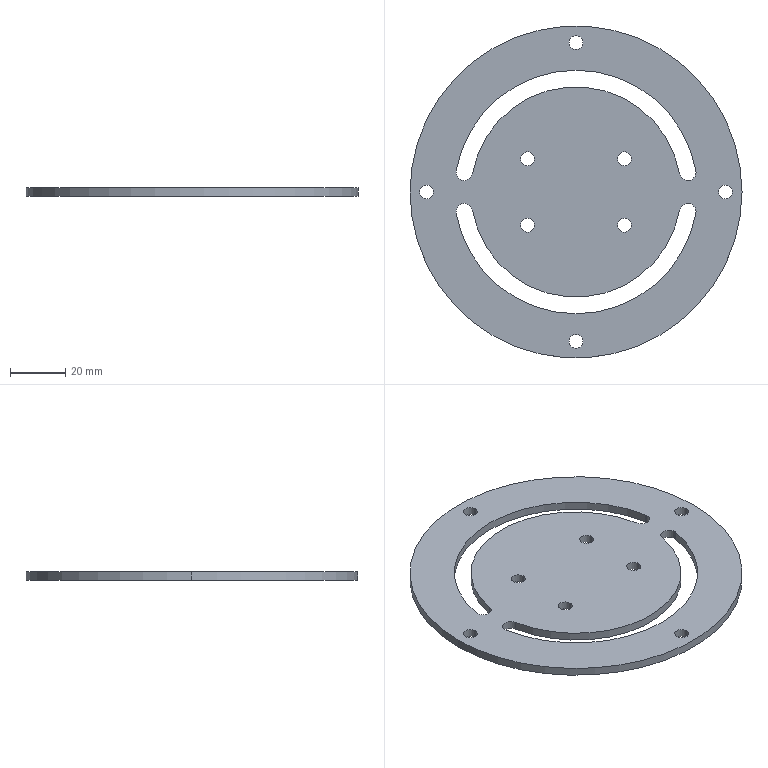Part | SolidWorks | features BaseBody 1 | 1 solid | 30 faces | box 120 x 120 x 3 mm | volume 29167 mm3 | cylinder 28 | plane 2 | commonest cylinder face diameters 5 x16 6 x6 76 x2 88 x2 120 x2
STEP:
#1=CARTESIAN_POINT('',(-60.,0.,3.));
#2=VERTEX_POINT('',#1);
#3=CARTESIAN_POINT('',(60.,0.,3.));
#4=VERTEX_POINT('',#3);
#5=CARTESIAN_POINT('',(0.,0.,3.));
#6=DIRECTION('',(0.,0.,-1.));
#7=DIRECTION('',(-1.,0.,0.));
#8=AXIS2_PLACEMENT_3D('',#5,#6,#7);
#9=CIRCLE('',#8,60.);
#10=EDGE_CURVE('',#2,#4,#9,.T.);
#11=ORIENTED_EDGE('',*,*,#10,.T.);
#12=CARTESIAN_POINT('',(60.,0.,0.));
#13=VERTEX_POINT('',#12);
#14=CARTESIAN_POINT('',(60.,0.,10.));
#15=DIRECTION('',(0.,0.,-1.));
#16=VECTOR('',#15,1000.);
#17=LINE('',#14,#16);
#18=EDGE_CURVE('',#4,#13,#17,.T.);
#19=ORIENTED_EDGE('',*,*,#18,.T.);
#20=CARTESIAN_POINT('',(-60.,0.,0.));
#21=VERTEX_POINT('',#20);
#22=CARTESIAN_POINT('',(0.,0.,0.));
#23=DIRECTION('',(0.,0.,-1.));
#24=DIRECTION('',(-1.,0.,0.));
#25=AXIS2_PLACEMENT_3D('',#22,#23,#24);
#26=CIRCLE('',#25,60.);
#27=EDGE_CURVE('',#21,#13,#26,.T.);
#28=ORIENTED_EDGE('',*,*,#27,.F.);
#29=CARTESIAN_POINT('',(-60.,0.,10.));
#30=DIRECTION('',(0.,0.,-1.));
#31=VECTOR('',#30,1000.);
#32=LINE('',#29,#31);
#33=EDGE_CURVE('',#2,#21,#32,.T.);
#34=ORIENTED_EDGE('',*,*,#33,.F.);
#35=EDGE_LOOP('',(#11,#19,#28,#34));
#36=FACE_OUTER_BOUND('',#35,.T.);
#37=CARTESIAN_POINT('',(0.,0.,10.));
#38=DIRECTION('',(0.,0.,-1.));
#39=DIRECTION('',(-1.,0.,0.));
#40=AXIS2_PLACEMENT_3D('',#37,#38,#39);
#41=CYLINDRICAL_SURFACE('',#40,60.);
#42=ADVANCED_FACE('',(#36),#41,.T.);
#43=CARTESIAN_POINT('',(43.377,7.12,0.));
#44=VERTEX_POINT('',#43);
#45=CARTESIAN_POINT('',(43.332,7.641,0.));
#46=VERTEX_POINT('',#45);
#47=CARTESIAN_POINT('',(40.377,7.12,0.));
#48=DIRECTION('',(0.,0.,1.));
#49=DIRECTION('',(1.,0.,0.));
#50=AXIS2_PLACEMENT_3D('',#47,#48,#49);
#51=CIRCLE('',#50,3.);
#52=EDGE_CURVE('',#44,#46,#51,.T.);
#53=ORIENTED_EDGE('',*,*,#52,.F.);
#54=CARTESIAN_POINT('',(43.377,7.12,3.));
#55=VERTEX_POINT('',#54);
#56=CARTESIAN_POINT('',(43.377,7.12,-7.));
#57=DIRECTION('',(0.,0.,1.));
#58=VECTOR('',#57,1000.);
#59=LINE('',#56,#58);
#60=EDGE_CURVE('',#44,#55,#59,.T.);
#61=ORIENTED_EDGE('',*,*,#60,.T.);
#62=CARTESIAN_POINT('',(43.332,7.641,3.));
#63=VERTEX_POINT('',#62);
#64=CARTESIAN_POINT('',(40.377,7.12,3.));
#65=DIRECTION('',(0.,0.,-1.));
#66=DIRECTION('',(1.,0.,0.));
#67=AXIS2_PLACEMENT_3D('',#64,#65,#66);
#68=CIRCLE('',#67,3.);
#69=EDGE_CURVE('',#63,#55,#68,.T.);
#70=ORIENTED_EDGE('',*,*,#69,.F.);
#71=CARTESIAN_POINT('',(43.332,7.641,-7.));
#72=DIRECTION('',(0.,0.,-1.));
#73=VECTOR('',#72,1000.);
#74=LINE('',#71,#73);
#75=EDGE_CURVE('',#63,#46,#74,.T.);
#76=ORIENTED_EDGE('',*,*,#75,.T.);
#77=EDGE_LOOP('',(#53,#61,#70,#76));
#78=FACE_OUTER_BOUND('',#77,.T.);
#79=CARTESIAN_POINT('',(40.377,7.12,-7.));
#80=DIRECTION('',(0.,0.,1.));
#81=DIRECTION('',(1.,0.,0.));
#82=AXIS2_PLACEMENT_3D('',#79,#80,#81);
#83=CYLINDRICAL_SURFACE('',#82,3.);
#84=ADVANCED_FACE('',(#78),#83,.F.);
#85=CARTESIAN_POINT('',(-15.,12.,3.));
#86=VERTEX_POINT('',#85);
#87=CARTESIAN_POINT('',(-20.,12.,3.));
#88=VERTEX_POINT('',#87);
#89=CARTESIAN_POINT('',(-17.5,12.,3.));
#90=DIRECTION('',(0.,0.,-1.));
#91=DIRECTION('',(-1.,0.,0.));
#92=AXIS2_PLACEMENT_3D('',#89,#90,#91);
#93=CIRCLE('',#92,2.5);
#94=EDGE_CURVE('',#86,#88,#93,.T.);
#95=ORIENTED_EDGE('',*,*,#94,.F.);
#96=CARTESIAN_POINT('',(-15.,12.,0.));
#97=VERTEX_POINT('',#96);
#98=CARTESIAN_POINT('',(-15.,12.,3.));
#99=DIRECTION('',(0.,0.,-1.));
#100=VECTOR('',#99,1000.);
#101=LINE('',#98,#100);
#102=EDGE_CURVE('',#86,#97,#101,.T.);
#103=ORIENTED_EDGE('',*,*,#102,.T.);
#104=CARTESIAN_POINT('',(-20.,12.,0.));
#105=VERTEX_POINT('',#104);
#106=CARTESIAN_POINT('',(-17.5,12.,0.));
#107=DIRECTION('',(0.,0.,1.));
#108=DIRECTION('',(-1.,0.,0.));
#109=AXIS2_PLACEMENT_3D('',#106,#107,#108);
#110=CIRCLE('',#109,2.5);
#111=EDGE_CURVE('',#105,#97,#110,.T.);
#112=ORIENTED_EDGE('',*,*,#111,.F.);
#113=CARTESIAN_POINT('',(-20.,12.,3.));
#114=DIRECTION('',(0.,0.,-1.));
#115=VECTOR('',#114,1000.);
#116=LINE('',#113,#115);
#117=EDGE_CURVE('',#88,#105,#116,.T.);
#118=ORIENTED_EDGE('',*,*,#117,.F.);
#119=EDGE_LOOP('',(#95,#103,#112,#118));
#120=FACE_OUTER_BOUND('',#119,.T.);
#121=CARTESIAN_POINT('',(-17.5,12.,3.));
#122=DIRECTION('',(0.,0.,-1.));
#123=DIRECTION('',(-1.,0.,0.));
#124=AXIS2_PLACEMENT_3D('',#121,#122,#123);
#125=CYLINDRICAL_SURFACE('',#124,2.5);
#126=ADVANCED_FACE('',(#120),#125,.F.);
#127=CARTESIAN_POINT('',(20.,-12.,3.));
#128=VERTEX_POINT('',#127);
#129=CARTESIAN_POINT('',(15.,-12.,3.));
#130=VERTEX_POINT('',#129);
#131=CARTESIAN_POINT('',(17.5,-12.,3.));
#132=DIRECTION('',(0.,0.,-1.));
#133=DIRECTION('',(-1.,0.,0.));
#134=AXIS2_PLACEMENT_3D('',#131,#132,#133);
#135=CIRCLE('',#134,2.5);
#136=EDGE_CURVE('',#128,#130,#135,.T.);
#137=ORIENTED_EDGE('',*,*,#136,.F.);
#138=CARTESIAN_POINT('',(20.,-12.,0.));
#139=VERTEX_POINT('',#138);
#140=CARTESIAN_POINT('',(20.,-12.,3.));
#141=DIRECTION('',(0.,0.,-1.));
#142=VECTOR('',#141,1000.);
#143=LINE('',#140,#142);
#144=EDGE_CURVE('',#128,#139,#143,.T.);
#145=ORIENTED_EDGE('',*,*,#144,.T.);
#146=CARTESIAN_POINT('',(15.,-12.,0.));
#147=VERTEX_POINT('',#146);
#148=CARTESIAN_POINT('',(17.5,-12.,0.));
#149=DIRECTION('',(0.,0.,1.));
#150=DIRECTION('',(-1.,0.,0.));
#151=AXIS2_PLACEMENT_3D('',#148,#149,#150);
#152=CIRCLE('',#151,2.5);
#153=EDGE_CURVE('',#147,#139,#152,.T.);
#154=ORIENTED_EDGE('',*,*,#153,.F.);
#155=CARTESIAN_POINT('',(15.,-12.,3.));
#156=DIRECTION('',(0.,0.,-1.));
#157=VECTOR('',#156,1000.);
#158=LINE('',#155,#157);
#159=EDGE_CURVE('',#130,#147,#158,.T.);
#160=ORIENTED_EDGE('',*,*,#159,.F.);
#161=EDGE_LOOP('',(#137,#145,#154,#160));
#162=FACE_OUTER_BOUND('',#161,.T.);
#163=CARTESIAN_POINT('',(17.5,-12.,3.));
#164=DIRECTION('',(0.,0.,-1.));
#165=DIRECTION('',(-1.,0.,0.));
#166=AXIS2_PLACEMENT_3D('',#163,#164,#165);
#167=CYLINDRICAL_SURFACE('',#166,2.5);
#168=ADVANCED_FACE('',(#162),#167,.F.);
#169=CARTESIAN_POINT('',(-51.5,0.,3.));
#170=VERTEX_POINT('',#169);
#171=CARTESIAN_POINT('',(-56.5,0.,3.));
#172=VERTEX_POINT('',#171);
#173=CARTESIAN_POINT('',(-54.,0.,3.));
#174=DIRECTION('',(0.,0.,-1.));
#175=DIRECTION('',(-1.,0.,0.));
#176=AXIS2_PLACEMENT_3D('',#173,#174,#175);
#177=CIRCLE('',#176,2.5);
#178=EDGE_CURVE('',#170,#172,#177,.T.);
#179=ORIENTED_EDGE('',*,*,#178,.F.);
#180=CARTESIAN_POINT('',(-51.5,0.,0.));
#181=VERTEX_POINT('',#180);
#182=CARTESIAN_POINT('',(-51.5,0.,3.));
#183=DIRECTION('',(0.,0.,-1.));
#184=VECTOR('',#183,1000.);
#185=LINE('',#182,#184);
#186=EDGE_CURVE('',#170,#181,#185,.T.);
#187=ORIENTED_EDGE('',*,*,#186,.T.);
#188=CARTESIAN_POINT('',(-56.5,0.,0.));
#189=VERTEX_POINT('',#188);
#190=CARTESIAN_POINT('',(-54.,0.,0.));
#191=DIRECTION('',(0.,0.,1.));
#192=DIRECTION('',(-1.,0.,0.));
#193=AXIS2_PLACEMENT_3D('',#190,#191,#192);
#194=CIRCLE('',#193,2.5);
#195=EDGE_CURVE('',#189,#181,#194,.T.);
#196=ORIENTED_EDGE('',*,*,#195,.F.);
#197=CARTESIAN_POINT('',(-56.5,0.,3.));
#198=DIRECTION('',(0.,0.,-1.));
#199=VECTOR('',#198,1000.);
#200=LINE('',#197,#199);
#201=EDGE_CURVE('',#172,#189,#200,.T.);
#202=ORIENTED_EDGE('',*,*,#201,.F.);
#203=EDGE_LOOP('',(#179,#187,#196,#202));
#204=FACE_OUTER_BOUND('',#203,.T.);
#205=CARTESIAN_POINT('',(-54.,0.,3.));
#206=DIRECTION('',(0.,0.,-1.));
#207=DIRECTION('',(-1.,0.,0.));
#208=AXIS2_PLACEMENT_3D('',#205,#206,#207);
#209=CYLINDRICAL_SURFACE('',#208,2.5);
#210=ADVANCED_FACE('',(#204),#209,.F.);
#211=CARTESIAN_POINT('',(56.5,0.,3.));
#212=VERTEX_POINT('',#211);
#213=CARTESIAN_POINT('',(51.5,0.,3.));
#214=VERTEX_POINT('',#213);
#215=CARTESIAN_POINT('',(54.,0.,3.));
#216=DIRECTION('',(0.,0.,-1.));
#217=DIRECTION('',(-1.,0.,0.));
#218=AXIS2_PLACEMENT_3D('',#215,#216,#217);
#219=CIRCLE('',#218,2.5);
#220=EDGE_CURVE('',#212,#214,#219,.T.);
#221=ORIENTED_EDGE('',*,*,#220,.F.);
#222=CARTESIAN_POINT('',(56.5,0.,0.));
#223=VERTEX_POINT('',#222);
#224=CARTESIAN_POINT('',(56.5,0.,3.));
#225=DIRECTION('',(0.,0.,-1.));
#226=VECTOR('',#225,1000.);
#227=LINE('',#224,#226);
#228=EDGE_CURVE('',#212,#223,#227,.T.);
#229=ORIENTED_EDGE('',*,*,#228,.T.);
#230=CARTESIAN_POINT('',(51.5,0.,0.));
#231=VERTEX_POINT('',#230);
#232=CARTESIAN_POINT('',(54.,0.,0.));
#233=DIRECTION('',(0.,0.,1.));
#234=DIRECTION('',(-1.,0.,0.));
#235=AXIS2_PLACEMENT_3D('',#232,#233,#234);
#236=CIRCLE('',#235,2.5);
#237=EDGE_CURVE('',#231,#223,#236,.T.);
#238=ORIENTED_EDGE('',*,*,#237,.F.);
#239=CARTESIAN_POINT('',(51.5,0.,3.));
#240=DIRECTION('',(0.,0.,-1.));
#241=VECTOR('',#240,1000.);
#242=LINE('',#239,#241);
#243=EDGE_CURVE('',#214,#231,#242,.T.);
#244=ORIENTED_EDGE('',*,*,#243,.F.);
#245=EDGE_LOOP('',(#221,#229,#238,#244));
#246=FACE_OUTER_BOUND('',#245,.T.);
#247=CARTESIAN_POINT('',(54.,0.,3.));
#248=DIRECTION('',(0.,0.,-1.));
#249=DIRECTION('',(-1.,0.,0.));
#250=AXIS2_PLACEMENT_3D('',#247,#248,#249);
#251=CYLINDRICAL_SURFACE('',#250,2.5);
#252=ADVANCED_FACE('',(#246),#251,.F.);
#253=CARTESIAN_POINT('',(2.5,54.,3.));
#254=VERTEX_POINT('',#253);
#255=CARTESIAN_POINT('',(-2.5,54.,3.));
#256=VERTEX_POINT('',#255);
#257=CARTESIAN_POINT('',(0.,54.,3.));
#258=DIRECTION('',(0.,0.,-1.));
#259=DIRECTION('',(-1.,0.,0.));
#260=AXIS2_PLACEMENT_3D('',#257,#258,#259);
#261=CIRCLE('',#260,2.5);
#262=EDGE_CURVE('',#254,#256,#261,.T.);
#263=ORIENTED_EDGE('',*,*,#262,.F.);
#264=CARTESIAN_POINT('',(2.5,54.,0.));
#265=VERTEX_POINT('',#264);
#266=CARTESIAN_POINT('',(2.5,54.,3.));
#267=DIRECTION('',(0.,0.,-1.));
#268=VECTOR('',#267,1000.);
#269=LINE('',#266,#268);
#270=EDGE_CURVE('',#254,#265,#269,.T.);
#271=ORIENTED_EDGE('',*,*,#270,.T.);
#272=CARTESIAN_POINT('',(-2.5,54.,0.));
#273=VERTEX_POINT('',#272);
#274=CARTESIAN_POINT('',(0.,54.,0.));
#275=DIRECTION('',(0.,0.,1.));
#276=DIRECTION('',(-1.,0.,0.));
#277=AXIS2_PLACEMENT_3D('',#274,#275,#276);
#278=CIRCLE('',#277,2.5);
#279=EDGE_CURVE('',#273,#265,#278,.T.);
#280=ORIENTED_EDGE('',*,*,#279,.F.);
#281=CARTESIAN_POINT('',(-2.5,54.,3.));
#282=DIRECTION('',(0.,0.,-1.));
#283=VECTOR('',#282,1000.);
#284=LINE('',#281,#283);
#285=EDGE_CURVE('',#256,#273,#284,.T.);
#286=ORIENTED_EDGE('',*,*,#285,.F.);
#287=EDGE_LOOP('',(#263,#271,#280,#286));
#288=FACE_OUTER_BOUND('',#287,.T.);
#289=CARTESIAN_POINT('',(0.,54.,3.));
#290=DIRECTION('',(0.,0.,-1.));
#291=DIRECTION('',(-1.,0.,0.));
#292=AXIS2_PLACEMENT_3D('',#289,#290,#291);
#293=CYLINDRICAL_SURFACE('',#292,2.5);
#294=ADVANCED_FACE('',(#288),#293,.F.);
#295=CARTESIAN_POINT('',(2.5,-54.,3.));
#296=VERTEX_POINT('',#295);
#297=CARTESIAN_POINT('',(-2.5,-54.,3.));
#298=VERTEX_POINT('',#297);
#299=CARTESIAN_POINT('',(0.,-54.,3.));
#300=DIRECTION('',(0.,0.,-1.));
#301=DIRECTION('',(-1.,0.,0.));
#302=AXIS2_PLACEMENT_3D('',#299,#300,#301);
#303=CIRCLE('',#302,2.5);
#304=EDGE_CURVE('',#296,#298,#303,.T.);
#305=ORIENTED_EDGE('',*,*,#304,.F.);
#306=CARTESIAN_POINT('',(2.5,-54.,0.));
#307=VERTEX_POINT('',#306);
#308=CARTESIAN_POINT('',(2.5,-54.,3.));
#309=DIRECTION('',(0.,0.,-1.));
#310=VECTOR('',#309,1000.);
#311=LINE('',#308,#310);
#312=EDGE_CURVE('',#296,#307,#311,.T.);
#313=ORIENTED_EDGE('',*,*,#312,.T.);
#314=CARTESIAN_POINT('',(-2.5,-54.,0.));
#315=VERTEX_POINT('',#314);
#316=CARTESIAN_POINT('',(0.,-54.,0.));
#317=DIRECTION('',(0.,0.,1.));
#318=DIRECTION('',(-1.,0.,0.));
#319=AXIS2_PLACEMENT_3D('',#316,#317,#318);
#320=CIRCLE('',#319,2.5);
#321=EDGE_CURVE('',#315,#307,#320,.T.);
#322=ORIENTED_EDGE('',*,*,#321,.F.);
#323=CARTESIAN_POINT('',(-2.5,-54.,3.));
#324=DIRECTION('',(0.,0.,-1.));
#325=VECTOR('',#324,1000.);
#326=LINE('',#323,#325);
#327=EDGE_CURVE('',#298,#315,#326,.T.);
#328=ORIENTED_EDGE('',*,*,#327,.F.);
#329=EDGE_LOOP('',(#305,#313,#322,#328));
#330=FACE_OUTER_BOUND('',#329,.T.);
#331=CARTESIAN_POINT('',(0.,-54.,3.));
#332=DIRECTION('',(0.,0.,-1.));
#333=DIRECTION('',(-1.,0.,0.));
#334=AXIS2_PLACEMENT_3D('',#331,#332,#333);
#335=CYLINDRICAL_SURFACE('',#334,2.5);
#336=ADVANCED_FACE('',(#330),#335,.F.);
#337=CARTESIAN_POINT('',(20.,12.,3.));
#338=VERTEX_POINT('',#337);
#339=CARTESIAN_POINT('',(15.,12.,3.));
#340=VERTEX_POINT('',#339);
#341=CARTESIAN_POINT('',(17.5,12.,3.));
#342=DIRECTION('',(0.,0.,-1.));
#343=DIRECTION('',(-1.,0.,0.));
#344=AXIS2_PLACEMENT_3D('',#341,#342,#343);
#345=CIRCLE('',#344,2.5);
#346=EDGE_CURVE('',#338,#340,#345,.T.);
#347=ORIENTED_EDGE('',*,*,#346,.F.);
#348=CARTESIAN_POINT('',(20.,12.,0.));
#349=VERTEX_POINT('',#348);
#350=CARTESIAN_POINT('',(20.,12.,3.));
#351=DIRECTION('',(0.,0.,-1.));
#352=VECTOR('',#351,1000.);
#353=LINE('',#350,#352);
#354=EDGE_CURVE('',#338,#349,#353,.T.);
#355=ORIENTED_EDGE('',*,*,#354,.T.);
#356=CARTESIAN_POINT('',(15.,12.,0.));
#357=VERTEX_POINT('',#356);
#358=CARTESIAN_POINT('',(17.5,12.,0.));
#359=DIRECTION('',(0.,0.,1.));
#360=DIRECTION('',(-1.,0.,0.));
#361=AXIS2_PLACEMENT_3D('',#358,#359,#360);
#362=CIRCLE('',#361,2.5);
#363=EDGE_CURVE('',#357,#349,#362,.T.);
#364=ORIENTED_EDGE('',*,*,#363,.F.);
#365=CARTESIAN_POINT('',(15.,12.,3.));
#366=DIRECTION('',(0.,0.,-1.));
#367=VECTOR('',#366,1000.);
#368=LINE('',#365,#367);
#369=EDGE_CURVE('',#340,#357,#368,.T.);
#370=ORIENTED_EDGE('',*,*,#369,.F.);
#371=EDGE_LOOP('',(#347,#355,#364,#370));
#372=FACE_OUTER_BOUND('',#371,.T.);
#373=CARTESIAN_POINT('',(17.5,12.,3.));
#374=DIRECTION('',(0.,0.,-1.));
#375=DIRECTION('',(-1.,0.,0.));
#376=AXIS2_PLACEMENT_3D('',#373,#374,#375);
#377=CYLINDRICAL_SURFACE('',#376,2.5);
#378=ADVANCED_FACE('',(#372),#377,.F.);
#379=CARTESIAN_POINT('',(-15.,-12.,3.));
#380=VERTEX_POINT('',#379);
#381=CARTESIAN_POINT('',(-20.,-12.,3.));
#382=VERTEX_POINT('',#381);
#383=CARTESIAN_POINT('',(-17.5,-12.,3.));
#384=DIRECTION('',(0.,0.,-1.));
#385=DIRECTION('',(-1.,0.,0.));
#386=AXIS2_PLACEMENT_3D('',#383,#384,#385);
#387=CIRCLE('',#386,2.5);
#388=EDGE_CURVE('',#380,#382,#387,.T.);
#389=ORIENTED_EDGE('',*,*,#388,.F.);
#390=CARTESIAN_POINT('',(-15.,-12.,0.));
#391=VERTEX_POINT('',#390);
#392=CARTESIAN_POINT('',(-15.,-12.,3.));
#393=DIRECTION('',(0.,0.,-1.));
#394=VECTOR('',#393,1000.);
#395=LINE('',#392,#394);
#396=EDGE_CURVE('',#380,#391,#395,.T.);
#397=ORIENTED_EDGE('',*,*,#396,.T.);
#398=CARTESIAN_POINT('',(-20.,-12.,0.));
#399=VERTEX_POINT('',#398);
#400=CARTESIAN_POINT('',(-17.5,-12.,0.));
#401=DIRECTION('',(0.,0.,1.));
#402=DIRECTION('',(-1.,0.,0.));
#403=AXIS2_PLACEMENT_3D('',#400,#401,#402);
#404=CIRCLE('',#403,2.5);
#405=EDGE_CURVE('',#399,#391,#404,.T.);
#406=ORIENTED_EDGE('',*,*,#405,.F.);
#407=CARTESIAN_POINT('',(-20.,-12.,3.));
#408=DIRECTION('',(0.,0.,-1.));
#409=VECTOR('',#408,1000.);
#410=LINE('',#407,#409);
#411=EDGE_CURVE('',#382,#399,#410,.T.);
#412=ORIENTED_EDGE('',*,*,#411,.F.);
#413=EDGE_LOOP('',(#389,#397,#406,#412));
#414=FACE_OUTER_BOUND('',#413,.T.);
#415=CARTESIAN_POINT('',(-17.5,-12.,3.));
#416=DIRECTION('',(0.,0.,-1.));
#417=DIRECTION('',(-1.,0.,0.));
#418=AXIS2_PLACEMENT_3D('',#415,#416,#417);
#419=CYLINDRICAL_SURFACE('',#418,2.5);
#420=ADVANCED_FACE('',(#414),#419,.F.);
#421=CARTESIAN_POINT('',(43.377,-7.12,0.));
#422=VERTEX_POINT('',#421);
#423=CARTESIAN_POINT('',(37.423,-6.599,0.));
#424=VERTEX_POINT('',#423);
#425=CARTESIAN_POINT('',(40.377,-7.12,0.));
#426=DIRECTION('',(0.,0.,1.));
#427=DIRECTION('',(1.,0.,0.));
#428=AXIS2_PLACEMENT_3D('',#425,#426,#427);
#429=CIRCLE('',#428,3.);
#430=EDGE_CURVE('',#422,#424,#429,.T.);
#431=ORIENTED_EDGE('',*,*,#430,.F.);
#432=CARTESIAN_POINT('',(43.377,-7.12,3.));
#433=VERTEX_POINT('',#432);
#434=CARTESIAN_POINT('',(43.377,-7.12,-7.));
#435=DIRECTION('',(0.,0.,1.));
#436=VECTOR('',#435,1000.);
#437=LINE('',#434,#436);
#438=EDGE_CURVE('',#422,#433,#437,.T.);
#439=ORIENTED_EDGE('',*,*,#438,.T.);
#440=CARTESIAN_POINT('',(37.423,-6.599,3.));
#441=VERTEX_POINT('',#440);
#442=CARTESIAN_POINT('',(40.377,-7.12,3.));
#443=DIRECTION('',(0.,0.,-1.));
#444=DIRECTION('',(1.,0.,0.));
#445=AXIS2_PLACEMENT_3D('',#442,#443,#444);
#446=CIRCLE('',#445,3.);
#447=EDGE_CURVE('',#441,#433,#446,.T.);
#448=ORIENTED_EDGE('',*,*,#447,.F.);
#449=CARTESIAN_POINT('',(37.423,-6.599,-7.));
#450=DIRECTION('',(0.,0.,1.));
#451=VECTOR('',#450,1000.);
#452=LINE('',#449,#451);
#453=EDGE_CURVE('',#424,#441,#452,.T.);
#454=ORIENTED_EDGE('',*,*,#453,.F.);
#455=EDGE_LOOP('',(#431,#439,#448,#454));
#456=FACE_OUTER_BOUND('',#455,.T.);
#457=CARTESIAN_POINT('',(40.377,-7.12,-7.));
#458=DIRECTION('',(0.,0.,1.));
#459=DIRECTION('',(1.,0.,0.));
#460=AXIS2_PLACEMENT_3D('',#457,#458,#459);
#461=CYLINDRICAL_SURFACE('',#460,3.);
#462=ADVANCED_FACE('',(#456),#461,.F.);
#463=ORIENTED_EDGE('',*,*,#27,.T.);
#464=CARTESIAN_POINT('',(0.,0.,0.));
#465=DIRECTION('',(0.,0.,-1.));
#466=DIRECTION('',(-1.,0.,0.));
#467=AXIS2_PLACEMENT_3D('',#464,#465,#466);
#468=CIRCLE('',#467,60.);
#469=EDGE_CURVE('',#13,#21,#468,.T.);
#470=ORIENTED_EDGE('',*,*,#469,.T.);
#471=EDGE_LOOP('',(#463,#470));
#472=FACE_OUTER_BOUND('',#471,.T.);
#473=CARTESIAN_POINT('',(-37.423,6.599,0.));
#474=VERTEX_POINT('',#473);
#475=CARTESIAN_POINT('',(37.423,6.599,0.));
#476=VERTEX_POINT('',#475);
#477=CARTESIAN_POINT('',(0.,0.,0.));
#478=DIRECTION('',(0.,0.,-1.));
#479=DIRECTION('',(1.,0.,0.));
#480=AXIS2_PLACEMENT_3D('',#477,#478,#479);
#481=CIRCLE('',#480,38.);
#482=EDGE_CURVE('',#474,#476,#481,.T.);
#483=ORIENTED_EDGE('',*,*,#482,.T.);
#484=CARTESIAN_POINT('',(40.377,7.12,0.));
#485=DIRECTION('',(0.,0.,1.));
#486=DIRECTION('',(1.,0.,0.));
#487=AXIS2_PLACEMENT_3D('',#484,#485,#486);
#488=CIRCLE('',#487,3.);
#489=EDGE_CURVE('',#476,#44,#488,.T.);
#490=ORIENTED_EDGE('',*,*,#489,.T.);
#491=ORIENTED_EDGE('',*,*,#52,.T.);
#492=CARTESIAN_POINT('',(-43.332,7.641,0.));
#493=VERTEX_POINT('',#492);
#494=CARTESIAN_POINT('',(0.,0.,0.));
#495=DIRECTION('',(0.,0.,1.));
#496=DIRECTION('',(1.,0.,0.));
#497=AXIS2_PLACEMENT_3D('',#494,#495,#496);
#498=CIRCLE('',#497,44.);
#499=EDGE_CURVE('',#46,#493,#498,.T.);
#500=ORIENTED_EDGE('',*,*,#499,.T.);
#501=CARTESIAN_POINT('',(-40.377,7.12,0.));
#502=DIRECTION('',(0.,0.,1.));
#503=DIRECTION('',(1.,0.,0.));
#504=AXIS2_PLACEMENT_3D('',#501,#502,#503);
#505=CIRCLE('',#504,3.);
#506=EDGE_CURVE('',#493,#474,#505,.T.);
#507=ORIENTED_EDGE('',*,*,#506,.T.);
#508=EDGE_LOOP('',(#483,#490,#491,#500,#507));
#509=FACE_BOUND('',#508,.T.);
#510=ORIENTED_EDGE('',*,*,#111,.T.);
#511=CARTESIAN_POINT('',(-17.5,12.,0.));
#512=DIRECTION('',(0.,0.,1.));
#513=DIRECTION('',(-1.,0.,0.));
#514=AXIS2_PLACEMENT_3D('',#511,#512,#513);
#515=CIRCLE('',#514,2.5);
#516=EDGE_CURVE('',#97,#105,#515,.T.);
#517=ORIENTED_EDGE('',*,*,#516,.T.);
#518=EDGE_LOOP('',(#510,#517));
#519=FACE_BOUND('',#518,.T.);
#520=ORIENTED_EDGE('',*,*,#153,.T.);
#521=CARTESIAN_POINT('',(17.5,-12.,0.));
#522=DIRECTION('',(0.,0.,1.));
#523=DIRECTION('',(-1.,0.,0.));
#524=AXIS2_PLACEMENT_3D('',#521,#522,#523);
#525=CIRCLE('',#524,2.5);
#526=EDGE_CURVE('',#139,#147,#525,.T.);
#527=ORIENTED_EDGE('',*,*,#526,.T.);
#528=EDGE_LOOP('',(#520,#527));
#529=FACE_BOUND('',#528,.T.);
#530=ORIENTED_EDGE('',*,*,#195,.T.);
#531=CARTESIAN_POINT('',(-54.,0.,0.));
#532=DIRECTION('',(0.,0.,1.));
#533=DIRECTION('',(-1.,0.,0.));
#534=AXIS2_PLACEMENT_3D('',#531,#532,#533);
#535=CIRCLE('',#534,2.5);
#536=EDGE_CURVE('',#181,#189,#535,.T.);
#537=ORIENTED_EDGE('',*,*,#536,.T.);
#538=EDGE_LOOP('',(#530,#537));
#539=FACE_BOUND('',#538,.T.);
#540=ORIENTED_EDGE('',*,*,#237,.T.);
#541=CARTESIAN_POINT('',(54.,0.,0.));
#542=DIRECTION('',(0.,0.,1.));
#543=DIRECTION('',(-1.,0.,0.));
#544=AXIS2_PLACEMENT_3D('',#541,#542,#543);
#545=CIRCLE('',#544,2.5);
#546=EDGE_CURVE('',#223,#231,#545,.T.);
#547=ORIENTED_EDGE('',*,*,#546,.T.);
#548=EDGE_LOOP('',(#540,#547));
#549=FACE_BOUND('',#548,.T.);
#550=ORIENTED_EDGE('',*,*,#279,.T.);
#551=CARTESIAN_POINT('',(0.,54.,0.));
#552=DIRECTION('',(0.,0.,1.));
#553=DIRECTION('',(-1.,0.,0.));
#554=AXIS2_PLACEMENT_3D('',#551,#552,#553);
#555=CIRCLE('',#554,2.5);
#556=EDGE_CURVE('',#265,#273,#555,.T.);
#557=ORIENTED_EDGE('',*,*,#556,.T.);
#558=EDGE_LOOP('',(#550,#557));
#559=FACE_BOUND('',#558,.T.);
#560=ORIENTED_EDGE('',*,*,#321,.T.);
#561=CARTESIAN_POINT('',(0.,-54.,0.));
#562=DIRECTION('',(0.,0.,1.));
#563=DIRECTION('',(-1.,0.,0.));
#564=AXIS2_PLACEMENT_3D('',#561,#562,#563);
#565=CIRCLE('',#564,2.5);
#566=EDGE_CURVE('',#307,#315,#565,.T.);
#567=ORIENTED_EDGE('',*,*,#566,.T.);
#568=EDGE_LOOP('',(#560,#567));
#569=FACE_BOUND('',#568,.T.);
#570=ORIENTED_EDGE('',*,*,#363,.T.);
#571=CARTESIAN_POINT('',(17.5,12.,0.));
#572=DIRECTION('',(0.,0.,1.));
#573=DIRECTION('',(-1.,0.,0.));
#574=AXIS2_PLACEMENT_3D('',#571,#572,#573);
#575=CIRCLE('',#574,2.5);
#576=EDGE_CURVE('',#349,#357,#575,.T.);
#577=ORIENTED_EDGE('',*,*,#576,.T.);
#578=EDGE_LOOP('',(#570,#577));
#579=FACE_BOUND('',#578,.T.);
#580=ORIENTED_EDGE('',*,*,#405,.T.);
#581=CARTESIAN_POINT('',(-17.5,-12.,0.));
#582=DIRECTION('',(0.,0.,1.));
#583=DIRECTION('',(-1.,0.,0.));
#584=AXIS2_PLACEMENT_3D('',#581,#582,#583);
#585=CIRCLE('',#584,2.5);
#586=EDGE_CURVE('',#391,#399,#585,.T.);
#587=ORIENTED_EDGE('',*,*,#586,.T.);
#588=EDGE_LOOP('',(#580,#587));
#589=FACE_BOUND('',#588,.T.);
#590=CARTESIAN_POINT('',(-43.332,-7.641,0.));
#591=VERTEX_POINT('',#590);
#592=CARTESIAN_POINT('',(43.332,-7.641,0.));
#593=VERTEX_POINT('',#592);
#594=CARTESIAN_POINT('',(0.,0.,0.));
#595=DIRECTION('',(0.,0.,1.));
#596=DIRECTION('',(1.,0.,0.));
#597=AXIS2_PLACEMENT_3D('',#594,#595,#596);
#598=CIRCLE('',#597,44.);
#599=EDGE_CURVE('',#591,#593,#598,.T.);
#600=ORIENTED_EDGE('',*,*,#599,.T.);
#601=CARTESIAN_POINT('',(40.377,-7.12,0.));
#602=DIRECTION('',(0.,0.,1.));
#603=DIRECTION('',(1.,0.,0.));
#604=AXIS2_PLACEMENT_3D('',#601,#602,#603);
#605=CIRCLE('',#604,3.);
#606=EDGE_CURVE('',#593,#422,#605,.T.);
#607=ORIENTED_EDGE('',*,*,#606,.T.);
#608=ORIENTED_EDGE('',*,*,#430,.T.);
#609=CARTESIAN_POINT('',(-37.423,-6.599,0.));
#610=VERTEX_POINT('',#609);
#611=CARTESIAN_POINT('',(0.,0.,0.));
#612=DIRECTION('',(0.,0.,-1.));
#613=DIRECTION('',(1.,0.,0.));
#614=AXIS2_PLACEMENT_3D('',#611,#612,#613);
#615=CIRCLE('',#614,38.);
#616=EDGE_CURVE('',#424,#610,#615,.T.);
#617=ORIENTED_EDGE('',*,*,#616,.T.);
#618=CARTESIAN_POINT('',(-40.377,-7.12,0.));
#619=DIRECTION('',(0.,0.,1.));
#620=DIRECTION('',(1.,0.,0.));
#621=AXIS2_PLACEMENT_3D('',#618,#619,#620);
#622=CIRCLE('',#621,3.);
#623=EDGE_CURVE('',#610,#591,#622,.T.);
#624=ORIENTED_EDGE('',*,*,#623,.T.);
#625=EDGE_LOOP('',(#600,#607,#608,#617,#624));
#626=FACE_BOUND('',#625,.T.);
#627=CARTESIAN_POINT('',(0.,0.,0.));
#628=DIRECTION('',(0.,0.,-1.));
#629=DIRECTION('',(-1.,0.,0.));
#630=AXIS2_PLACEMENT_3D('',#627,#628,#629);
#631=PLANE('',#630);
#632=ADVANCED_FACE('',(#472,#509,#519,#529,#539,#549,#559,#569,#579,#589,#626),#631,.T.);
#633=ORIENTED_EDGE('',*,*,#18,.F.);
#634=CARTESIAN_POINT('',(0.,0.,3.));
#635=DIRECTION('',(0.,0.,-1.));
#636=DIRECTION('',(-1.,0.,0.));
#637=AXIS2_PLACEMENT_3D('',#634,#635,#636);
#638=CIRCLE('',#637,60.);
#639=EDGE_CURVE('',#4,#2,#638,.T.);
#640=ORIENTED_EDGE('',*,*,#639,.T.);
#641=ORIENTED_EDGE('',*,*,#33,.T.);
#642=ORIENTED_EDGE('',*,*,#469,.F.);
#643=EDGE_LOOP('',(#633,#640,#641,#642));
#644=FACE_OUTER_BOUND('',#643,.T.);
#645=CARTESIAN_POINT('',(0.,0.,10.));
#646=DIRECTION('',(0.,0.,-1.));
#647=DIRECTION('',(-1.,0.,0.));
#648=AXIS2_PLACEMENT_3D('',#645,#646,#647);
#649=CYLINDRICAL_SURFACE('',#648,60.);
#650=ADVANCED_FACE('',(#644),#649,.T.);
#651=ORIENTED_EDGE('',*,*,#60,.F.);
#652=ORIENTED_EDGE('',*,*,#489,.F.);
#653=CARTESIAN_POINT('',(37.423,6.599,3.));
#654=VERTEX_POINT('',#653);
#655=CARTESIAN_POINT('',(37.423,6.599,-7.));
#656=DIRECTION('',(0.,0.,-1.));
#657=VECTOR('',#656,1000.);
#658=LINE('',#655,#657);
#659=EDGE_CURVE('',#654,#476,#658,.T.);
#660=ORIENTED_EDGE('',*,*,#659,.F.);
#661=CARTESIAN_POINT('',(40.377,7.12,3.));
#662=DIRECTION('',(0.,0.,-1.));
#663=DIRECTION('',(1.,0.,0.));
#664=AXIS2_PLACEMENT_3D('',#661,#662,#663);
#665=CIRCLE('',#664,3.);
#666=EDGE_CURVE('',#55,#654,#665,.T.);
#667=ORIENTED_EDGE('',*,*,#666,.F.);
#668=EDGE_LOOP('',(#651,#652,#660,#667));
#669=FACE_OUTER_BOUND('',#668,.T.);
#670=CARTESIAN_POINT('',(40.377,7.12,-7.));
#671=DIRECTION('',(0.,0.,1.));
#672=DIRECTION('',(1.,0.,0.));
#673=AXIS2_PLACEMENT_3D('',#670,#671,#672);
#674=CYLINDRICAL_SURFACE('',#673,3.);
#675=ADVANCED_FACE('',(#669),#674,.F.);
#676=CARTESIAN_POINT('',(-37.423,6.599,3.));
#677=VERTEX_POINT('',#676);
#678=CARTESIAN_POINT('',(0.,0.,3.));
#679=DIRECTION('',(0.,0.,-1.));
#680=DIRECTION('',(1.,0.,0.));
#681=AXIS2_PLACEMENT_3D('',#678,#679,#680);
#682=CIRCLE('',#681,38.);
#683=EDGE_CURVE('',#677,#654,#682,.T.);
#684=ORIENTED_EDGE('',*,*,#683,.T.);
#685=ORIENTED_EDGE('',*,*,#659,.T.);
#686=ORIENTED_EDGE('',*,*,#482,.F.);
#687=CARTESIAN_POINT('',(-37.423,6.599,-7.));
#688=DIRECTION('',(0.,0.,1.));
#689=VECTOR('',#688,1000.);
#690=LINE('',#687,#689);
#691=EDGE_CURVE('',#474,#677,#690,.T.);
#692=ORIENTED_EDGE('',*,*,#691,.T.);
#693=EDGE_LOOP('',(#684,#685,#686,#692));
#694=FACE_OUTER_BOUND('',#693,.T.);
#695=CARTESIAN_POINT('',(0.,0.,-7.));
#696=DIRECTION('',(0.,0.,1.));
#697=DIRECTION('',(1.,0.,0.));
#698=AXIS2_PLACEMENT_3D('',#695,#696,#697);
#699=CYLINDRICAL_SURFACE('',#698,38.);
#700=ADVANCED_FACE('',(#694),#699,.T.);
#701=CARTESIAN_POINT('',(-43.332,7.641,3.));
#702=VERTEX_POINT('',#701);
#703=CARTESIAN_POINT('',(-43.332,7.641,-7.));
#704=DIRECTION('',(0.,0.,-1.));
#705=VECTOR('',#704,1000.);
#706=LINE('',#703,#705);
#707=EDGE_CURVE('',#702,#493,#706,.T.);
#708=ORIENTED_EDGE('',*,*,#707,.F.);
#709=CARTESIAN_POINT('',(-40.377,7.12,3.));
#710=DIRECTION('',(0.,0.,-1.));
#711=DIRECTION('',(1.,0.,0.));
#712=AXIS2_PLACEMENT_3D('',#709,#710,#711);
#713=CIRCLE('',#712,3.);
#714=EDGE_CURVE('',#677,#702,#713,.T.);
#715=ORIENTED_EDGE('',*,*,#714,.F.);
#716=ORIENTED_EDGE('',*,*,#691,.F.);
#717=ORIENTED_EDGE('',*,*,#506,.F.);
#718=EDGE_LOOP('',(#708,#715,#716,#717));
#719=FACE_OUTER_BOUND('',#718,.T.);
#720=CARTESIAN_POINT('',(-40.377,7.12,-7.));
#721=DIRECTION('',(0.,0.,1.));
#722=DIRECTION('',(1.,0.,0.));
#723=AXIS2_PLACEMENT_3D('',#720,#721,#722);
#724=CYLINDRICAL_SURFACE('',#723,3.);
#725=ADVANCED_FACE('',(#719),#724,.F.);
#726=ORIENTED_EDGE('',*,*,#75,.F.);
#727=CARTESIAN_POINT('',(0.,0.,3.));
#728=DIRECTION('',(0.,0.,-1.));
#729=DIRECTION('',(1.,0.,0.));
#730=AXIS2_PLACEMENT_3D('',#727,#728,#729);
#731=CIRCLE('',#730,44.);
#732=EDGE_CURVE('',#702,#63,#731,.T.);
#733=ORIENTED_EDGE('',*,*,#732,.F.);
#734=ORIENTED_EDGE('',*,*,#707,.T.);
#735=ORIENTED_EDGE('',*,*,#499,.F.);
#736=EDGE_LOOP('',(#726,#733,#734,#735));
#737=FACE_OUTER_BOUND('',#736,.T.);
#738=CARTESIAN_POINT('',(0.,0.,-7.));
#739=DIRECTION('',(0.,0.,1.));
#740=DIRECTION('',(1.,0.,0.));
#741=AXIS2_PLACEMENT_3D('',#738,#739,#740);
#742=CYLINDRICAL_SURFACE('',#741,44.);
#743=ADVANCED_FACE('',(#737),#742,.F.);
#744=ORIENTED_EDGE('',*,*,#102,.F.);
#745=CARTESIAN_POINT('',(-17.5,12.,3.));
#746=DIRECTION('',(0.,0.,-1.));
#747=DIRECTION('',(-1.,0.,0.));
#748=AXIS2_PLACEMENT_3D('',#745,#746,#747);
#749=CIRCLE('',#748,2.5);
#750=EDGE_CURVE('',#88,#86,#749,.T.);
#751=ORIENTED_EDGE('',*,*,#750,.F.);
#752=ORIENTED_EDGE('',*,*,#117,.T.);
#753=ORIENTED_EDGE('',*,*,#516,.F.);
#754=EDGE_LOOP('',(#744,#751,#752,#753));
#755=FACE_OUTER_BOUND('',#754,.T.);
#756=CARTESIAN_POINT('',(-17.5,12.,3.));
#757=DIRECTION('',(0.,0.,-1.));
#758=DIRECTION('',(-1.,0.,0.));
#759=AXIS2_PLACEMENT_3D('',#756,#757,#758);
#760=CYLINDRICAL_SURFACE('',#759,2.5);
#761=ADVANCED_FACE('',(#755),#760,.F.);
#762=ORIENTED_EDGE('',*,*,#144,.F.);
#763=CARTESIAN_POINT('',(17.5,-12.,3.));
#764=DIRECTION('',(0.,0.,-1.));
#765=DIRECTION('',(-1.,0.,0.));
#766=AXIS2_PLACEMENT_3D('',#763,#764,#765);
#767=CIRCLE('',#766,2.5);
#768=EDGE_CURVE('',#130,#128,#767,.T.);
#769=ORIENTED_EDGE('',*,*,#768,.F.);
#770=ORIENTED_EDGE('',*,*,#159,.T.);
#771=ORIENTED_EDGE('',*,*,#526,.F.);
#772=EDGE_LOOP('',(#762,#769,#770,#771));
#773=FACE_OUTER_BOUND('',#772,.T.);
#774=CARTESIAN_POINT('',(17.5,-12.,3.));
#775=DIRECTION('',(0.,0.,-1.));
#776=DIRECTION('',(-1.,0.,0.));
#777=AXIS2_PLACEMENT_3D('',#774,#775,#776);
#778=CYLINDRICAL_SURFACE('',#777,2.5);
#779=ADVANCED_FACE('',(#773),#778,.F.);
#780=ORIENTED_EDGE('',*,*,#186,.F.);
#781=CARTESIAN_POINT('',(-54.,0.,3.));
#782=DIRECTION('',(0.,0.,-1.));
#783=DIRECTION('',(-1.,0.,0.));
#784=AXIS2_PLACEMENT_3D('',#781,#782,#783);
#785=CIRCLE('',#784,2.5);
#786=EDGE_CURVE('',#172,#170,#785,.T.);
#787=ORIENTED_EDGE('',*,*,#786,.F.);
#788=ORIENTED_EDGE('',*,*,#201,.T.);
#789=ORIENTED_EDGE('',*,*,#536,.F.);
#790=EDGE_LOOP('',(#780,#787,#788,#789));
#791=FACE_OUTER_BOUND('',#790,.T.);
#792=CARTESIAN_POINT('',(-54.,0.,3.));
#793=DIRECTION('',(0.,0.,-1.));
#794=DIRECTION('',(-1.,0.,0.));
#795=AXIS2_PLACEMENT_3D('',#792,#793,#794);
#796=CYLINDRICAL_SURFACE('',#795,2.5);
#797=ADVANCED_FACE('',(#791),#796,.F.);
#798=ORIENTED_EDGE('',*,*,#228,.F.);
#799=CARTESIAN_POINT('',(54.,0.,3.));
#800=DIRECTION('',(0.,0.,-1.));
#801=DIRECTION('',(-1.,0.,0.));
#802=AXIS2_PLACEMENT_3D('',#799,#800,#801);
#803=CIRCLE('',#802,2.5);
#804=EDGE_CURVE('',#214,#212,#803,.T.);
#805=ORIENTED_EDGE('',*,*,#804,.F.);
#806=ORIENTED_EDGE('',*,*,#243,.T.);
#807=ORIENTED_EDGE('',*,*,#546,.F.);
#808=EDGE_LOOP('',(#798,#805,#806,#807));
#809=FACE_OUTER_BOUND('',#808,.T.);
#810=CARTESIAN_POINT('',(54.,0.,3.));
#811=DIRECTION('',(0.,0.,-1.));
#812=DIRECTION('',(-1.,0.,0.));
#813=AXIS2_PLACEMENT_3D('',#810,#811,#812);
#814=CYLINDRICAL_SURFACE('',#813,2.5);
#815=ADVANCED_FACE('',(#809),#814,.F.);
#816=ORIENTED_EDGE('',*,*,#270,.F.);
#817=CARTESIAN_POINT('',(0.,54.,3.));
#818=DIRECTION('',(0.,0.,-1.));
#819=DIRECTION('',(-1.,0.,0.));
#820=AXIS2_PLACEMENT_3D('',#817,#818,#819);
#821=CIRCLE('',#820,2.5);
#822=EDGE_CURVE('',#256,#254,#821,.T.);
#823=ORIENTED_EDGE('',*,*,#822,.F.);
#824=ORIENTED_EDGE('',*,*,#285,.T.);
#825=ORIENTED_EDGE('',*,*,#556,.F.);
#826=EDGE_LOOP('',(#816,#823,#824,#825));
#827=FACE_OUTER_BOUND('',#826,.T.);
#828=CARTESIAN_POINT('',(0.,54.,3.));
#829=DIRECTION('',(0.,0.,-1.));
#830=DIRECTION('',(-1.,0.,0.));
#831=AXIS2_PLACEMENT_3D('',#828,#829,#830);
#832=CYLINDRICAL_SURFACE('',#831,2.5);
#833=ADVANCED_FACE('',(#827),#832,.F.);
#834=ORIENTED_EDGE('',*,*,#312,.F.);
#835=CARTESIAN_POINT('',(0.,-54.,3.));
#836=DIRECTION('',(0.,0.,-1.));
#837=DIRECTION('',(-1.,0.,0.));
#838=AXIS2_PLACEMENT_3D('',#835,#836,#837);
#839=CIRCLE('',#838,2.5);
#840=EDGE_CURVE('',#298,#296,#839,.T.);
#841=ORIENTED_EDGE('',*,*,#840,.F.);
#842=ORIENTED_EDGE('',*,*,#327,.T.);
#843=ORIENTED_EDGE('',*,*,#566,.F.);
#844=EDGE_LOOP('',(#834,#841,#842,#843));
#845=FACE_OUTER_BOUND('',#844,.T.);
#846=CARTESIAN_POINT('',(0.,-54.,3.));
#847=DIRECTION('',(0.,0.,-1.));
#848=DIRECTION('',(-1.,0.,0.));
#849=AXIS2_PLACEMENT_3D('',#846,#847,#848);
#850=CYLINDRICAL_SURFACE('',#849,2.5);
#851=ADVANCED_FACE('',(#845),#850,.F.);
#852=ORIENTED_EDGE('',*,*,#354,.F.);
#853=CARTESIAN_POINT('',(17.5,12.,3.));
#854=DIRECTION('',(0.,0.,-1.));
#855=DIRECTION('',(-1.,0.,0.));
#856=AXIS2_PLACEMENT_3D('',#853,#854,#855);
#857=CIRCLE('',#856,2.5);
#858=EDGE_CURVE('',#340,#338,#857,.T.);
#859=ORIENTED_EDGE('',*,*,#858,.F.);
#860=ORIENTED_EDGE('',*,*,#369,.T.);
#861=ORIENTED_EDGE('',*,*,#576,.F.);
#862=EDGE_LOOP('',(#852,#859,#860,#861));
#863=FACE_OUTER_BOUND('',#862,.T.);
#864=CARTESIAN_POINT('',(17.5,12.,3.));
#865=DIRECTION('',(0.,0.,-1.));
#866=DIRECTION('',(-1.,0.,0.));
#867=AXIS2_PLACEMENT_3D('',#864,#865,#866);
#868=CYLINDRICAL_SURFACE('',#867,2.5);
#869=ADVANCED_FACE('',(#863),#868,.F.);
#870=ORIENTED_EDGE('',*,*,#396,.F.);
#871=CARTESIAN_POINT('',(-17.5,-12.,3.));
#872=DIRECTION('',(0.,0.,-1.));
#873=DIRECTION('',(-1.,0.,0.));
#874=AXIS2_PLACEMENT_3D('',#871,#872,#873);
#875=CIRCLE('',#874,2.5);
#876=EDGE_CURVE('',#382,#380,#875,.T.);
#877=ORIENTED_EDGE('',*,*,#876,.F.);
#878=ORIENTED_EDGE('',*,*,#411,.T.);
#879=ORIENTED_EDGE('',*,*,#586,.F.);
#880=EDGE_LOOP('',(#870,#877,#878,#879));
#881=FACE_OUTER_BOUND('',#880,.T.);
#882=CARTESIAN_POINT('',(-17.5,-12.,3.));
#883=DIRECTION('',(0.,0.,-1.));
#884=DIRECTION('',(-1.,0.,0.));
#885=AXIS2_PLACEMENT_3D('',#882,#883,#884);
#886=CYLINDRICAL_SURFACE('',#885,2.5);
#887=ADVANCED_FACE('',(#881),#886,.F.);
#888=CARTESIAN_POINT('',(-43.332,-7.641,3.));
#889=VERTEX_POINT('',#888);
#890=CARTESIAN_POINT('',(-43.332,-7.641,-7.));
#891=DIRECTION('',(0.,0.,-1.));
#892=VECTOR('',#891,1000.);
#893=LINE('',#890,#892);
#894=EDGE_CURVE('',#889,#591,#893,.T.);
#895=ORIENTED_EDGE('',*,*,#894,.F.);
#896=CARTESIAN_POINT('',(43.332,-7.641,3.));
#897=VERTEX_POINT('',#896);
#898=CARTESIAN_POINT('',(0.,0.,3.));
#899=DIRECTION('',(0.,0.,-1.));
#900=DIRECTION('',(1.,0.,0.));
#901=AXIS2_PLACEMENT_3D('',#898,#899,#900);
#902=CIRCLE('',#901,44.);
#903=EDGE_CURVE('',#897,#889,#902,.T.);
#904=ORIENTED_EDGE('',*,*,#903,.F.);
#905=CARTESIAN_POINT('',(43.332,-7.641,-7.));
#906=DIRECTION('',(0.,0.,1.));
#907=VECTOR('',#906,1000.);
#908=LINE('',#905,#907);
#909=EDGE_CURVE('',#593,#897,#908,.T.);
#910=ORIENTED_EDGE('',*,*,#909,.F.);
#911=ORIENTED_EDGE('',*,*,#599,.F.);
#912=EDGE_LOOP('',(#895,#904,#910,#911));
#913=FACE_OUTER_BOUND('',#912,.T.);
#914=CARTESIAN_POINT('',(0.,0.,-7.));
#915=DIRECTION('',(0.,0.,1.));
#916=DIRECTION('',(1.,0.,0.));
#917=AXIS2_PLACEMENT_3D('',#914,#915,#916);
#918=CYLINDRICAL_SURFACE('',#917,44.);
#919=ADVANCED_FACE('',(#913),#918,.F.);
#920=CARTESIAN_POINT('',(-37.423,-6.599,3.));
#921=VERTEX_POINT('',#920);
#922=CARTESIAN_POINT('',(-37.423,-6.599,-7.));
#923=DIRECTION('',(0.,0.,-1.));
#924=VECTOR('',#923,1000.);
#925=LINE('',#922,#924);
#926=EDGE_CURVE('',#921,#610,#925,.T.);
#927=ORIENTED_EDGE('',*,*,#926,.F.);
#928=CARTESIAN_POINT('',(-40.377,-7.12,3.));
#929=DIRECTION('',(0.,0.,-1.));
#930=DIRECTION('',(1.,0.,0.));
#931=AXIS2_PLACEMENT_3D('',#928,#929,#930);
#932=CIRCLE('',#931,3.);
#933=EDGE_CURVE('',#889,#921,#932,.T.);
#934=ORIENTED_EDGE('',*,*,#933,.F.);
#935=ORIENTED_EDGE('',*,*,#894,.T.);
#936=ORIENTED_EDGE('',*,*,#623,.F.);
#937=EDGE_LOOP('',(#927,#934,#935,#936));
#938=FACE_OUTER_BOUND('',#937,.T.);
#939=CARTESIAN_POINT('',(-40.377,-7.12,-7.));
#940=DIRECTION('',(0.,0.,1.));
#941=DIRECTION('',(1.,0.,0.));
#942=AXIS2_PLACEMENT_3D('',#939,#940,#941);
#943=CYLINDRICAL_SURFACE('',#942,3.);
#944=ADVANCED_FACE('',(#938),#943,.F.);
#945=CARTESIAN_POINT('',(0.,0.,3.));
#946=DIRECTION('',(0.,0.,-1.));
#947=DIRECTION('',(1.,0.,0.));
#948=AXIS2_PLACEMENT_3D('',#945,#946,#947);
#949=CIRCLE('',#948,38.);
#950=EDGE_CURVE('',#441,#921,#949,.T.);
#951=ORIENTED_EDGE('',*,*,#950,.T.);
#952=ORIENTED_EDGE('',*,*,#926,.T.);
#953=ORIENTED_EDGE('',*,*,#616,.F.);
#954=ORIENTED_EDGE('',*,*,#453,.T.);
#955=EDGE_LOOP('',(#951,#952,#953,#954));
#956=FACE_OUTER_BOUND('',#955,.T.);
#957=CARTESIAN_POINT('',(0.,0.,-7.));
#958=DIRECTION('',(0.,0.,1.));
#959=DIRECTION('',(1.,0.,0.));
#960=AXIS2_PLACEMENT_3D('',#957,#958,#959);
#961=CYLINDRICAL_SURFACE('',#960,38.);
#962=ADVANCED_FACE('',(#956),#961,.T.);
#963=ORIENTED_EDGE('',*,*,#438,.F.);
#964=ORIENTED_EDGE('',*,*,#606,.F.);
#965=ORIENTED_EDGE('',*,*,#909,.T.);
#966=CARTESIAN_POINT('',(40.377,-7.12,3.));
#967=DIRECTION('',(0.,0.,-1.));
#968=DIRECTION('',(1.,0.,0.));
#969=AXIS2_PLACEMENT_3D('',#966,#967,#968);
#970=CIRCLE('',#969,3.);
#971=EDGE_CURVE('',#433,#897,#970,.T.);
#972=ORIENTED_EDGE('',*,*,#971,.F.);
#973=EDGE_LOOP('',(#963,#964,#965,#972));
#974=FACE_OUTER_BOUND('',#973,.T.);
#975=CARTESIAN_POINT('',(40.377,-7.12,-7.));
#976=DIRECTION('',(0.,0.,1.));
#977=DIRECTION('',(1.,0.,0.));
#978=AXIS2_PLACEMENT_3D('',#975,#976,#977);
#979=CYLINDRICAL_SURFACE('',#978,3.);
#980=ADVANCED_FACE('',(#974),#979,.F.);
#981=ORIENTED_EDGE('',*,*,#10,.F.);
#982=ORIENTED_EDGE('',*,*,#639,.F.);
#983=EDGE_LOOP('',(#981,#982));
#984=FACE_OUTER_BOUND('',#983,.T.);
#985=ORIENTED_EDGE('',*,*,#732,.T.);
#986=ORIENTED_EDGE('',*,*,#69,.T.);
#987=ORIENTED_EDGE('',*,*,#666,.T.);
#988=ORIENTED_EDGE('',*,*,#683,.F.);
#989=ORIENTED_EDGE('',*,*,#714,.T.);
#990=EDGE_LOOP('',(#985,#986,#987,#988,#989));
#991=FACE_BOUND('',#990,.T.);
#992=ORIENTED_EDGE('',*,*,#447,.T.);
#993=ORIENTED_EDGE('',*,*,#971,.T.);
#994=ORIENTED_EDGE('',*,*,#903,.T.);
#995=ORIENTED_EDGE('',*,*,#933,.T.);
#996=ORIENTED_EDGE('',*,*,#950,.F.);
#997=EDGE_LOOP('',(#992,#993,#994,#995,#996));
#998=FACE_BOUND('',#997,.T.);
#999=ORIENTED_EDGE('',*,*,#750,.T.);
#1000=ORIENTED_EDGE('',*,*,#94,.T.);
#1001=EDGE_LOOP('',(#999,#1000));
#1002=FACE_BOUND('',#1001,.T.);
#1003=ORIENTED_EDGE('',*,*,#876,.T.);
#1004=ORIENTED_EDGE('',*,*,#388,.T.);
#1005=EDGE_LOOP('',(#1003,#1004));
#1006=FACE_BOUND('',#1005,.T.);
#1007=ORIENTED_EDGE('',*,*,#768,.T.);
#1008=ORIENTED_EDGE('',*,*,#136,.T.);
#1009=EDGE_LOOP('',(#1007,#1008));
#1010=FACE_BOUND('',#1009,.T.);
#1011=ORIENTED_EDGE('',*,*,#858,.T.);
#1012=ORIENTED_EDGE('',*,*,#346,.T.);
#1013=EDGE_LOOP('',(#1011,#1012));
#1014=FACE_BOUND('',#1013,.T.);
#1015=ORIENTED_EDGE('',*,*,#786,.T.);
#1016=ORIENTED_EDGE('',*,*,#178,.T.);
#1017=EDGE_LOOP('',(#1015,#1016));
#1018=FACE_BOUND('',#1017,.T.);
#1019=ORIENTED_EDGE('',*,*,#840,.T.);
#1020=ORIENTED_EDGE('',*,*,#304,.T.);
#1021=EDGE_LOOP('',(#1019,#1020));
#1022=FACE_BOUND('',#1021,.T.);
#1023=ORIENTED_EDGE('',*,*,#804,.T.);
#1024=ORIENTED_EDGE('',*,*,#220,.T.);
#1025=EDGE_LOOP('',(#1023,#1024));
#1026=FACE_BOUND('',#1025,.T.);
#1027=ORIENTED_EDGE('',*,*,#822,.T.);
#1028=ORIENTED_EDGE('',*,*,#262,.T.);
#1029=EDGE_LOOP('',(#1027,#1028));
#1030=FACE_BOUND('',#1029,.T.);
#1031=CARTESIAN_POINT('',(0.,0.,3.));
#1032=DIRECTION('',(0.,0.,-1.));
#1033=DIRECTION('',(-1.,0.,0.));
#1034=AXIS2_PLACEMENT_3D('',#1031,#1032,#1033);
#1035=PLANE('',#1034);
#1036=ADVANCED_FACE('',(#984,#991,#998,#1002,#1006,#1010,#1014,#1018,#1022,#1026,#1030),#1035,.F.);
#1037=CLOSED_SHELL('',(#42,#84,#126,#168,#210,#252,#294,#336,#378,#420,#462,#632,#650,#675,#700,#725,#743,#761,#779,#797,#815,#833,#851,#869,#887,#919,#944,#962,#980,#1036));
#1038=MANIFOLD_SOLID_BREP('',#1037);
#1039=CARTESIAN_POINT('',(0.,0.,0.));
#1040=DIRECTION('',(0.,0.,1.));
#1041=DIRECTION('',(1.,0.,0.));
#1042=AXIS2_PLACEMENT_3D('',#1039,#1040,#1041);
#1043=(LENGTH_UNIT()NAMED_UNIT(*)SI_UNIT(.MILLI.,.METRE.));
#1044=UNCERTAINTY_MEASURE_WITH_UNIT(LENGTH_MEASURE(0.00001),#1043,'','');
#1045=(NAMED_UNIT(*)PLANE_ANGLE_UNIT()SI_UNIT($,.RADIAN.));
#1046=(NAMED_UNIT(*)SI_UNIT($,.STERADIAN.)SOLID_ANGLE_UNIT());
#1047=(GEOMETRIC_REPRESENTATION_CONTEXT(3)GLOBAL_UNCERTAINTY_ASSIGNED_CONTEXT((#1044))GLOBAL_UNIT_ASSIGNED_CONTEXT((#1043,#1045,#1046))REPRESENTATION_CONTEXT('',''));
#1048=ADVANCED_BREP_SHAPE_REPRESENTATION('',(#1038,#1042),#1047);